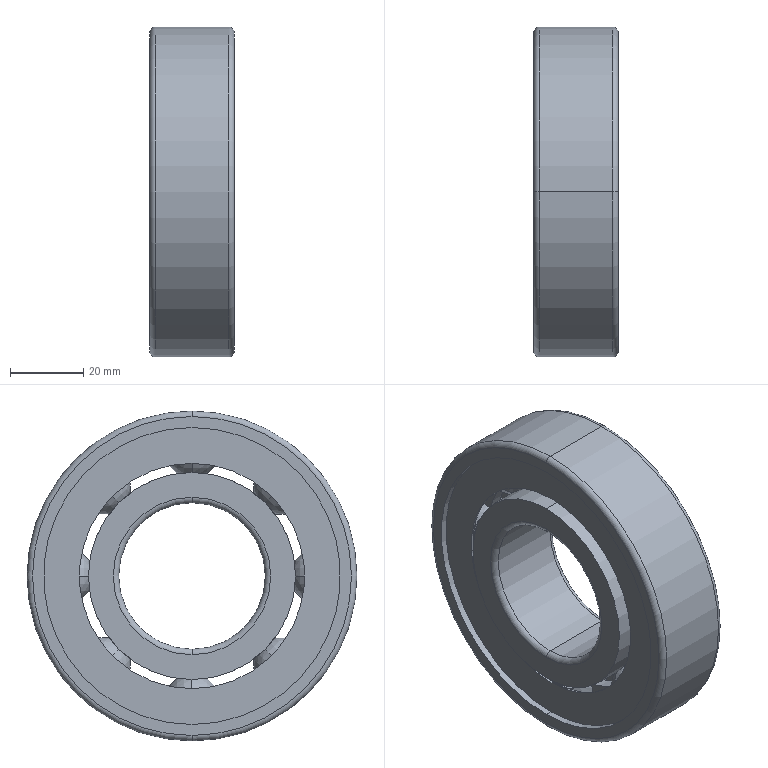Part | STEP file | GB/T276-94 deep groove ball bearing 6308-2Z | 1 solid | 144 faces | box 23 x 90 x 90 mm | volume 71674 mm3 | sphere 64 | torus 32 | cylinder 24 | plane 24 | commonest cylinder face diameters 81 x8 56.5 x4 61.477 x4 40 x2 64.603 x2 72.897 x2